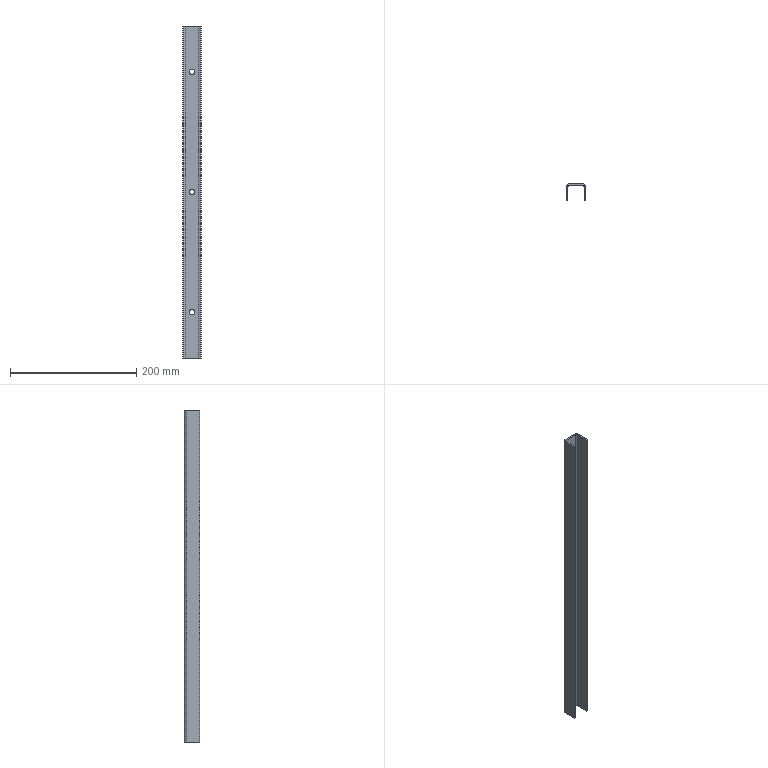Part | STEP file | SYL_0392D6J1SYL0380DJ10-1341050 | 1 solid | 28 faces | box 30 x 25 x 525 mm | volume 76794 mm3 | plane 18 | cylinder 10 | commonest cylinder face diameters 8 x8 4 x2
STEP:
#1=CARTESIAN_POINT('',(0.,23.,-194.));
#2=VERTEX_POINT('',#1);
#3=CARTESIAN_POINT('',(0.,25.,-194.));
#4=VERTEX_POINT('',#3);
#5=CARTESIAN_POINT('',(0.,25.,-194.));
#6=DIRECTION('',(0.,1.,0.));
#7=VECTOR('',#6,1000.);
#8=LINE('',#5,#7);
#9=EDGE_CURVE('',#2,#4,#8,.T.);
#10=ORIENTED_EDGE('',*,*,#9,.F.);
#11=CARTESIAN_POINT('',(0.,23.,-186.));
#12=VERTEX_POINT('',#11);
#13=CARTESIAN_POINT('',(0.,23.,-190.));
#14=DIRECTION('',(0.,-1.,0.));
#15=DIRECTION('',(0.,0.,-1.));
#16=AXIS2_PLACEMENT_3D('',#13,#14,#15);
#17=CIRCLE('',#16,4.);
#18=EDGE_CURVE('',#2,#12,#17,.T.);
#19=ORIENTED_EDGE('',*,*,#18,.T.);
#20=CARTESIAN_POINT('',(0.,25.,-186.));
#21=VERTEX_POINT('',#20);
#22=CARTESIAN_POINT('',(0.,25.,-186.));
#23=DIRECTION('',(0.,1.,0.));
#24=VECTOR('',#23,1000.);
#25=LINE('',#22,#24);
#26=EDGE_CURVE('',#12,#21,#25,.T.);
#27=ORIENTED_EDGE('',*,*,#26,.T.);
#28=CARTESIAN_POINT('',(0.,25.,-190.));
#29=DIRECTION('',(0.,-1.,0.));
#30=DIRECTION('',(0.,0.,-1.));
#31=AXIS2_PLACEMENT_3D('',#28,#29,#30);
#32=CIRCLE('',#31,4.);
#33=EDGE_CURVE('',#4,#21,#32,.T.);
#34=ORIENTED_EDGE('',*,*,#33,.F.);
#35=EDGE_LOOP('',(#10,#19,#27,#34));
#36=FACE_OUTER_BOUND('',#35,.T.);
#37=CARTESIAN_POINT('',(0.,25.,-190.));
#38=DIRECTION('',(0.,1.,0.));
#39=DIRECTION('',(0.,0.,1.));
#40=AXIS2_PLACEMENT_3D('',#37,#38,#39);
#41=CYLINDRICAL_SURFACE('',#40,4.);
#42=ADVANCED_FACE('',(#36),#41,.F.);
#43=CARTESIAN_POINT('',(0.,23.,-4.));
#44=VERTEX_POINT('',#43);
#45=CARTESIAN_POINT('',(0.,25.,-4.));
#46=VERTEX_POINT('',#45);
#47=CARTESIAN_POINT('',(0.,25.,-4.));
#48=DIRECTION('',(0.,1.,0.));
#49=VECTOR('',#48,1000.);
#50=LINE('',#47,#49);
#51=EDGE_CURVE('',#44,#46,#50,.T.);
#52=ORIENTED_EDGE('',*,*,#51,.F.);
#53=CARTESIAN_POINT('',(0.,23.,4.));
#54=VERTEX_POINT('',#53);
#55=CARTESIAN_POINT('',(0.,23.,0.));
#56=DIRECTION('',(0.,-1.,0.));
#57=DIRECTION('',(0.,0.,-1.));
#58=AXIS2_PLACEMENT_3D('',#55,#56,#57);
#59=CIRCLE('',#58,4.);
#60=EDGE_CURVE('',#44,#54,#59,.T.);
#61=ORIENTED_EDGE('',*,*,#60,.T.);
#62=CARTESIAN_POINT('',(0.,25.,4.));
#63=VERTEX_POINT('',#62);
#64=CARTESIAN_POINT('',(0.,25.,4.));
#65=DIRECTION('',(0.,1.,0.));
#66=VECTOR('',#65,1000.);
#67=LINE('',#64,#66);
#68=EDGE_CURVE('',#54,#63,#67,.T.);
#69=ORIENTED_EDGE('',*,*,#68,.T.);
#70=CARTESIAN_POINT('',(0.,25.,0.));
#71=DIRECTION('',(0.,-1.,0.));
#72=DIRECTION('',(0.,0.,-1.));
#73=AXIS2_PLACEMENT_3D('',#70,#71,#72);
#74=CIRCLE('',#73,4.);
#75=EDGE_CURVE('',#46,#63,#74,.T.);
#76=ORIENTED_EDGE('',*,*,#75,.F.);
#77=EDGE_LOOP('',(#52,#61,#69,#76));
#78=FACE_OUTER_BOUND('',#77,.T.);
#79=CARTESIAN_POINT('',(0.,25.,0.));
#80=DIRECTION('',(0.,1.,0.));
#81=DIRECTION('',(0.,0.,1.));
#82=AXIS2_PLACEMENT_3D('',#79,#80,#81);
#83=CYLINDRICAL_SURFACE('',#82,4.);
#84=ADVANCED_FACE('',(#78),#83,.F.);
#85=CARTESIAN_POINT('',(0.,23.,186.));
#86=VERTEX_POINT('',#85);
#87=CARTESIAN_POINT('',(0.,25.,186.));
#88=VERTEX_POINT('',#87);
#89=CARTESIAN_POINT('',(0.,25.,186.));
#90=DIRECTION('',(0.,1.,0.));
#91=VECTOR('',#90,1000.);
#92=LINE('',#89,#91);
#93=EDGE_CURVE('',#86,#88,#92,.T.);
#94=ORIENTED_EDGE('',*,*,#93,.F.);
#95=CARTESIAN_POINT('',(0.,23.,194.));
#96=VERTEX_POINT('',#95);
#97=CARTESIAN_POINT('',(0.,23.,190.));
#98=DIRECTION('',(0.,-1.,0.));
#99=DIRECTION('',(0.,0.,-1.));
#100=AXIS2_PLACEMENT_3D('',#97,#98,#99);
#101=CIRCLE('',#100,4.);
#102=EDGE_CURVE('',#86,#96,#101,.T.);
#103=ORIENTED_EDGE('',*,*,#102,.T.);
#104=CARTESIAN_POINT('',(0.,25.,194.));
#105=VERTEX_POINT('',#104);
#106=CARTESIAN_POINT('',(0.,25.,194.));
#107=DIRECTION('',(0.,1.,0.));
#108=VECTOR('',#107,1000.);
#109=LINE('',#106,#108);
#110=EDGE_CURVE('',#96,#105,#109,.T.);
#111=ORIENTED_EDGE('',*,*,#110,.T.);
#112=CARTESIAN_POINT('',(0.,25.,190.));
#113=DIRECTION('',(0.,-1.,0.));
#114=DIRECTION('',(0.,0.,-1.));
#115=AXIS2_PLACEMENT_3D('',#112,#113,#114);
#116=CIRCLE('',#115,4.);
#117=EDGE_CURVE('',#88,#105,#116,.T.);
#118=ORIENTED_EDGE('',*,*,#117,.F.);
#119=EDGE_LOOP('',(#94,#103,#111,#118));
#120=FACE_OUTER_BOUND('',#119,.T.);
#121=CARTESIAN_POINT('',(0.,25.,190.));
#122=DIRECTION('',(0.,1.,0.));
#123=DIRECTION('',(0.,0.,1.));
#124=AXIS2_PLACEMENT_3D('',#121,#122,#123);
#125=CYLINDRICAL_SURFACE('',#124,4.);
#126=ADVANCED_FACE('',(#120),#125,.F.);
#127=CARTESIAN_POINT('',(-11.,23.,-262.5));
#128=VERTEX_POINT('',#127);
#129=CARTESIAN_POINT('',(-11.,25.,-262.5));
#130=VERTEX_POINT('',#129);
#131=CARTESIAN_POINT('',(-11.,25.,-262.5));
#132=DIRECTION('',(0.,1.,0.));
#133=VECTOR('',#132,1000.);
#134=LINE('',#131,#133);
#135=EDGE_CURVE('',#128,#130,#134,.T.);
#136=ORIENTED_EDGE('',*,*,#135,.F.);
#137=CARTESIAN_POINT('',(-13.,21.,-262.5));
#138=VERTEX_POINT('',#137);
#139=CARTESIAN_POINT('',(-11.,21.,-262.5));
#140=DIRECTION('',(0.,0.,-1.));
#141=DIRECTION('',(1.,0.,0.));
#142=AXIS2_PLACEMENT_3D('',#139,#140,#141);
#143=CIRCLE('',#142,2.);
#144=EDGE_CURVE('',#138,#128,#143,.T.);
#145=ORIENTED_EDGE('',*,*,#144,.F.);
#146=CARTESIAN_POINT('',(-15.,21.,-262.5));
#147=VERTEX_POINT('',#146);
#148=CARTESIAN_POINT('',(-15.,21.,-262.5));
#149=DIRECTION('',(-1.,0.,0.));
#150=VECTOR('',#149,1000.);
#151=LINE('',#148,#150);
#152=EDGE_CURVE('',#138,#147,#151,.T.);
#153=ORIENTED_EDGE('',*,*,#152,.T.);
#154=CARTESIAN_POINT('',(-11.,21.,-262.5));
#155=DIRECTION('',(0.,0.,-1.));
#156=DIRECTION('',(-1.,0.,0.));
#157=AXIS2_PLACEMENT_3D('',#154,#155,#156);
#158=CIRCLE('',#157,4.);
#159=EDGE_CURVE('',#147,#130,#158,.T.);
#160=ORIENTED_EDGE('',*,*,#159,.T.);
#161=EDGE_LOOP('',(#136,#145,#153,#160));
#162=FACE_OUTER_BOUND('',#161,.T.);
#163=CARTESIAN_POINT('',(-11.,21.,-262.5));
#164=DIRECTION('',(0.,0.,1.));
#165=DIRECTION('',(1.,0.,0.));
#166=AXIS2_PLACEMENT_3D('',#163,#164,#165);
#167=PLANE('',#166);
#168=ADVANCED_FACE('',(#162),#167,.F.);
#169=ORIENTED_EDGE('',*,*,#152,.F.);
#170=CARTESIAN_POINT('',(-13.,0.,-262.5));
#171=VERTEX_POINT('',#170);
#172=CARTESIAN_POINT('',(-13.,21.,-262.5));
#173=DIRECTION('',(0.,-1.,0.));
#174=VECTOR('',#173,1000.);
#175=LINE('',#172,#174);
#176=EDGE_CURVE('',#138,#171,#175,.T.);
#177=ORIENTED_EDGE('',*,*,#176,.T.);
#178=CARTESIAN_POINT('',(-15.,0.,-262.5));
#179=VERTEX_POINT('',#178);
#180=CARTESIAN_POINT('',(-15.,0.,-262.5));
#181=DIRECTION('',(-1.,0.,0.));
#182=VECTOR('',#181,1000.);
#183=LINE('',#180,#182);
#184=EDGE_CURVE('',#171,#179,#183,.T.);
#185=ORIENTED_EDGE('',*,*,#184,.T.);
#186=CARTESIAN_POINT('',(-15.,21.,-262.5));
#187=DIRECTION('',(0.,-1.,0.));
#188=VECTOR('',#187,1000.);
#189=LINE('',#186,#188);
#190=EDGE_CURVE('',#147,#179,#189,.T.);
#191=ORIENTED_EDGE('',*,*,#190,.F.);
#192=EDGE_LOOP('',(#169,#177,#185,#191));
#193=FACE_OUTER_BOUND('',#192,.T.);
#194=CARTESIAN_POINT('',(-15.,21.,-262.5));
#195=DIRECTION('',(0.,0.,-1.));
#196=DIRECTION('',(0.,-1.,0.));
#197=AXIS2_PLACEMENT_3D('',#194,#195,#196);
#198=PLANE('',#197);
#199=ADVANCED_FACE('',(#193),#198,.T.);
#200=ORIENTED_EDGE('',*,*,#184,.F.);
#201=CARTESIAN_POINT('',(-13.,0.,262.5));
#202=VERTEX_POINT('',#201);
#203=CARTESIAN_POINT('',(-13.,0.,-262.5));
#204=DIRECTION('',(0.,0.,1.));
#205=VECTOR('',#204,1000.);
#206=LINE('',#203,#205);
#207=EDGE_CURVE('',#171,#202,#206,.T.);
#208=ORIENTED_EDGE('',*,*,#207,.T.);
#209=CARTESIAN_POINT('',(-15.,0.,262.5));
#210=VERTEX_POINT('',#209);
#211=CARTESIAN_POINT('',(-15.,0.,262.5));
#212=DIRECTION('',(-1.,0.,0.));
#213=VECTOR('',#212,1000.);
#214=LINE('',#211,#213);
#215=EDGE_CURVE('',#202,#210,#214,.T.);
#216=ORIENTED_EDGE('',*,*,#215,.T.);
#217=CARTESIAN_POINT('',(-15.,0.,-262.5));
#218=DIRECTION('',(0.,0.,1.));
#219=VECTOR('',#218,1000.);
#220=LINE('',#217,#219);
#221=EDGE_CURVE('',#179,#210,#220,.T.);
#222=ORIENTED_EDGE('',*,*,#221,.F.);
#223=EDGE_LOOP('',(#200,#208,#216,#222));
#224=FACE_OUTER_BOUND('',#223,.T.);
#225=CARTESIAN_POINT('',(-15.,0.,-262.5));
#226=DIRECTION('',(0.,-1.,0.));
#227=DIRECTION('',(0.,0.,1.));
#228=AXIS2_PLACEMENT_3D('',#225,#226,#227);
#229=PLANE('',#228);
#230=ADVANCED_FACE('',(#224),#229,.T.);
#231=ORIENTED_EDGE('',*,*,#215,.F.);
#232=CARTESIAN_POINT('',(-13.,21.,262.5));
#233=VERTEX_POINT('',#232);
#234=CARTESIAN_POINT('',(-13.,21.,262.5));
#235=DIRECTION('',(0.,-1.,0.));
#236=VECTOR('',#235,1000.);
#237=LINE('',#234,#236);
#238=EDGE_CURVE('',#233,#202,#237,.T.);
#239=ORIENTED_EDGE('',*,*,#238,.F.);
#240=CARTESIAN_POINT('',(-15.,21.,262.5));
#241=VERTEX_POINT('',#240);
#242=CARTESIAN_POINT('',(-15.,21.,262.5));
#243=DIRECTION('',(-1.,0.,0.));
#244=VECTOR('',#243,1000.);
#245=LINE('',#242,#244);
#246=EDGE_CURVE('',#233,#241,#245,.T.);
#247=ORIENTED_EDGE('',*,*,#246,.T.);
#248=CARTESIAN_POINT('',(-15.,21.,262.5));
#249=DIRECTION('',(0.,-1.,0.));
#250=VECTOR('',#249,1000.);
#251=LINE('',#248,#250);
#252=EDGE_CURVE('',#241,#210,#251,.T.);
#253=ORIENTED_EDGE('',*,*,#252,.T.);
#254=EDGE_LOOP('',(#231,#239,#247,#253));
#255=FACE_OUTER_BOUND('',#254,.T.);
#256=CARTESIAN_POINT('',(-15.,21.,262.5));
#257=DIRECTION('',(0.,0.,-1.));
#258=DIRECTION('',(0.,-1.,0.));
#259=AXIS2_PLACEMENT_3D('',#256,#257,#258);
#260=PLANE('',#259);
#261=ADVANCED_FACE('',(#255),#260,.F.);
#262=ORIENTED_EDGE('',*,*,#246,.F.);
#263=CARTESIAN_POINT('',(-11.,23.,262.5));
#264=VERTEX_POINT('',#263);
#265=CARTESIAN_POINT('',(-11.,21.,262.5));
#266=DIRECTION('',(0.,0.,1.));
#267=DIRECTION('',(1.,0.,0.));
#268=AXIS2_PLACEMENT_3D('',#265,#266,#267);
#269=CIRCLE('',#268,2.);
#270=EDGE_CURVE('',#264,#233,#269,.T.);
#271=ORIENTED_EDGE('',*,*,#270,.F.);
#272=CARTESIAN_POINT('',(-11.,25.,262.5));
#273=VERTEX_POINT('',#272);
#274=CARTESIAN_POINT('',(-11.,25.,262.5));
#275=DIRECTION('',(0.,1.,0.));
#276=VECTOR('',#275,1000.);
#277=LINE('',#274,#276);
#278=EDGE_CURVE('',#264,#273,#277,.T.);
#279=ORIENTED_EDGE('',*,*,#278,.T.);
#280=CARTESIAN_POINT('',(-11.,21.,262.5));
#281=DIRECTION('',(0.,0.,1.));
#282=DIRECTION('',(0.,1.,0.));
#283=AXIS2_PLACEMENT_3D('',#280,#281,#282);
#284=CIRCLE('',#283,4.);
#285=EDGE_CURVE('',#273,#241,#284,.T.);
#286=ORIENTED_EDGE('',*,*,#285,.T.);
#287=EDGE_LOOP('',(#262,#271,#279,#286));
#288=FACE_OUTER_BOUND('',#287,.T.);
#289=CARTESIAN_POINT('',(-11.,21.,262.5));
#290=DIRECTION('',(0.,0.,-1.));
#291=DIRECTION('',(-1.,0.,0.));
#292=AXIS2_PLACEMENT_3D('',#289,#290,#291);
#293=PLANE('',#292);
#294=ADVANCED_FACE('',(#288),#293,.F.);
#295=ORIENTED_EDGE('',*,*,#278,.F.);
#296=CARTESIAN_POINT('',(11.,23.,262.5));
#297=VERTEX_POINT('',#296);
#298=CARTESIAN_POINT('',(11.,23.,262.5));
#299=DIRECTION('',(-1.,0.,0.));
#300=VECTOR('',#299,1000.);
#301=LINE('',#298,#300);
#302=EDGE_CURVE('',#297,#264,#301,.T.);
#303=ORIENTED_EDGE('',*,*,#302,.F.);
#304=CARTESIAN_POINT('',(11.,25.,262.5));
#305=VERTEX_POINT('',#304);
#306=CARTESIAN_POINT('',(11.,25.,262.5));
#307=DIRECTION('',(0.,1.,0.));
#308=VECTOR('',#307,1000.);
#309=LINE('',#306,#308);
#310=EDGE_CURVE('',#297,#305,#309,.T.);
#311=ORIENTED_EDGE('',*,*,#310,.T.);
#312=CARTESIAN_POINT('',(11.,25.,262.5));
#313=DIRECTION('',(-1.,0.,0.));
#314=VECTOR('',#313,1000.);
#315=LINE('',#312,#314);
#316=EDGE_CURVE('',#305,#273,#315,.T.);
#317=ORIENTED_EDGE('',*,*,#316,.T.);
#318=EDGE_LOOP('',(#295,#303,#311,#317));
#319=FACE_OUTER_BOUND('',#318,.T.);
#320=CARTESIAN_POINT('',(11.,25.,262.5));
#321=DIRECTION('',(0.,0.,-1.));
#322=DIRECTION('',(-1.,0.,0.));
#323=AXIS2_PLACEMENT_3D('',#320,#321,#322);
#324=PLANE('',#323);
#325=ADVANCED_FACE('',(#319),#324,.F.);
#326=ORIENTED_EDGE('',*,*,#310,.F.);
#327=CARTESIAN_POINT('',(13.,21.,262.5));
#328=VERTEX_POINT('',#327);
#329=CARTESIAN_POINT('',(11.,21.,262.5));
#330=DIRECTION('',(0.,0.,1.));
#331=DIRECTION('',(1.,0.,0.));
#332=AXIS2_PLACEMENT_3D('',#329,#330,#331);
#333=CIRCLE('',#332,2.);
#334=EDGE_CURVE('',#328,#297,#333,.T.);
#335=ORIENTED_EDGE('',*,*,#334,.F.);
#336=CARTESIAN_POINT('',(15.,21.,262.5));
#337=VERTEX_POINT('',#336);
#338=CARTESIAN_POINT('',(15.,21.,262.5));
#339=DIRECTION('',(1.,0.,0.));
#340=VECTOR('',#339,1000.);
#341=LINE('',#338,#340);
#342=EDGE_CURVE('',#328,#337,#341,.T.);
#343=ORIENTED_EDGE('',*,*,#342,.T.);
#344=CARTESIAN_POINT('',(11.,21.,262.5));
#345=DIRECTION('',(0.,0.,1.));
#346=DIRECTION('',(1.,0.,0.));
#347=AXIS2_PLACEMENT_3D('',#344,#345,#346);
#348=CIRCLE('',#347,4.);
#349=EDGE_CURVE('',#337,#305,#348,.T.);
#350=ORIENTED_EDGE('',*,*,#349,.T.);
#351=EDGE_LOOP('',(#326,#335,#343,#350));
#352=FACE_OUTER_BOUND('',#351,.T.);
#353=CARTESIAN_POINT('',(11.,21.,262.5));
#354=DIRECTION('',(0.,0.,-1.));
#355=DIRECTION('',(-1.,0.,0.));
#356=AXIS2_PLACEMENT_3D('',#353,#354,#355);
#357=PLANE('',#356);
#358=ADVANCED_FACE('',(#352),#357,.F.);
#359=ORIENTED_EDGE('',*,*,#342,.F.);
#360=CARTESIAN_POINT('',(13.,0.,262.5));
#361=VERTEX_POINT('',#360);
#362=CARTESIAN_POINT('',(13.,0.,262.5));
#363=DIRECTION('',(0.,1.,0.));
#364=VECTOR('',#363,1000.);
#365=LINE('',#362,#364);
#366=EDGE_CURVE('',#361,#328,#365,.T.);
#367=ORIENTED_EDGE('',*,*,#366,.F.);
#368=CARTESIAN_POINT('',(15.,0.,262.5));
#369=VERTEX_POINT('',#368);
#370=CARTESIAN_POINT('',(15.,0.,262.5));
#371=DIRECTION('',(1.,0.,0.));
#372=VECTOR('',#371,1000.);
#373=LINE('',#370,#372);
#374=EDGE_CURVE('',#361,#369,#373,.T.);
#375=ORIENTED_EDGE('',*,*,#374,.T.);
#376=CARTESIAN_POINT('',(15.,0.,262.5));
#377=DIRECTION('',(0.,1.,0.));
#378=VECTOR('',#377,1000.);
#379=LINE('',#376,#378);
#380=EDGE_CURVE('',#369,#337,#379,.T.);
#381=ORIENTED_EDGE('',*,*,#380,.T.);
#382=EDGE_LOOP('',(#359,#367,#375,#381));
#383=FACE_OUTER_BOUND('',#382,.T.);
#384=CARTESIAN_POINT('',(15.,0.,262.5));
#385=DIRECTION('',(0.,0.,-1.));
#386=DIRECTION('',(0.,1.,0.));
#387=AXIS2_PLACEMENT_3D('',#384,#385,#386);
#388=PLANE('',#387);
#389=ADVANCED_FACE('',(#383),#388,.F.);
#390=ORIENTED_EDGE('',*,*,#374,.F.);
#391=CARTESIAN_POINT('',(13.,0.,-262.5));
#392=VERTEX_POINT('',#391);
#393=CARTESIAN_POINT('',(13.,0.,-262.5));
#394=DIRECTION('',(0.,0.,1.));
#395=VECTOR('',#394,1000.);
#396=LINE('',#393,#395);
#397=EDGE_CURVE('',#392,#361,#396,.T.);
#398=ORIENTED_EDGE('',*,*,#397,.F.);
#399=CARTESIAN_POINT('',(15.,0.,-262.5));
#400=VERTEX_POINT('',#399);
#401=CARTESIAN_POINT('',(15.,0.,-262.5));
#402=DIRECTION('',(1.,0.,0.));
#403=VECTOR('',#402,1000.);
#404=LINE('',#401,#403);
#405=EDGE_CURVE('',#392,#400,#404,.T.);
#406=ORIENTED_EDGE('',*,*,#405,.T.);
#407=CARTESIAN_POINT('',(15.,0.,-262.5));
#408=DIRECTION('',(0.,0.,1.));
#409=VECTOR('',#408,1000.);
#410=LINE('',#407,#409);
#411=EDGE_CURVE('',#400,#369,#410,.T.);
#412=ORIENTED_EDGE('',*,*,#411,.T.);
#413=EDGE_LOOP('',(#390,#398,#406,#412));
#414=FACE_OUTER_BOUND('',#413,.T.);
#415=CARTESIAN_POINT('',(15.,0.,-262.5));
#416=DIRECTION('',(0.,1.,0.));
#417=DIRECTION('',(0.,0.,1.));
#418=AXIS2_PLACEMENT_3D('',#415,#416,#417);
#419=PLANE('',#418);
#420=ADVANCED_FACE('',(#414),#419,.F.);
#421=ORIENTED_EDGE('',*,*,#405,.F.);
#422=CARTESIAN_POINT('',(13.,21.,-262.5));
#423=VERTEX_POINT('',#422);
#424=CARTESIAN_POINT('',(13.,0.,-262.5));
#425=DIRECTION('',(0.,1.,0.));
#426=VECTOR('',#425,1000.);
#427=LINE('',#424,#426);
#428=EDGE_CURVE('',#392,#423,#427,.T.);
#429=ORIENTED_EDGE('',*,*,#428,.T.);
#430=CARTESIAN_POINT('',(15.,21.,-262.5));
#431=VERTEX_POINT('',#430);
#432=CARTESIAN_POINT('',(15.,21.,-262.5));
#433=DIRECTION('',(1.,0.,0.));
#434=VECTOR('',#433,1000.);
#435=LINE('',#432,#434);
#436=EDGE_CURVE('',#423,#431,#435,.T.);
#437=ORIENTED_EDGE('',*,*,#436,.T.);
#438=CARTESIAN_POINT('',(15.,0.,-262.5));
#439=DIRECTION('',(0.,1.,0.));
#440=VECTOR('',#439,1000.);
#441=LINE('',#438,#440);
#442=EDGE_CURVE('',#400,#431,#441,.T.);
#443=ORIENTED_EDGE('',*,*,#442,.F.);
#444=EDGE_LOOP('',(#421,#429,#437,#443));
#445=FACE_OUTER_BOUND('',#444,.T.);
#446=CARTESIAN_POINT('',(15.,0.,-262.5));
#447=DIRECTION('',(0.,0.,-1.));
#448=DIRECTION('',(0.,1.,0.));
#449=AXIS2_PLACEMENT_3D('',#446,#447,#448);
#450=PLANE('',#449);
#451=ADVANCED_FACE('',(#445),#450,.T.);
#452=ORIENTED_EDGE('',*,*,#436,.F.);
#453=CARTESIAN_POINT('',(11.,23.,-262.5));
#454=VERTEX_POINT('',#453);
#455=CARTESIAN_POINT('',(11.,21.,-262.5));
#456=DIRECTION('',(0.,0.,-1.));
#457=DIRECTION('',(1.,0.,0.));
#458=AXIS2_PLACEMENT_3D('',#455,#456,#457);
#459=CIRCLE('',#458,2.);
#460=EDGE_CURVE('',#454,#423,#459,.T.);
#461=ORIENTED_EDGE('',*,*,#460,.F.);
#462=CARTESIAN_POINT('',(11.,25.,-262.5));
#463=VERTEX_POINT('',#462);
#464=CARTESIAN_POINT('',(11.,25.,-262.5));
#465=DIRECTION('',(0.,1.,0.));
#466=VECTOR('',#465,1000.);
#467=LINE('',#464,#466);
#468=EDGE_CURVE('',#454,#463,#467,.T.);
#469=ORIENTED_EDGE('',*,*,#468,.T.);
#470=CARTESIAN_POINT('',(11.,21.,-262.5));
#471=DIRECTION('',(0.,0.,-1.));
#472=DIRECTION('',(0.,1.,0.));
#473=AXIS2_PLACEMENT_3D('',#470,#471,#472);
#474=CIRCLE('',#473,4.);
#475=EDGE_CURVE('',#463,#431,#474,.T.);
#476=ORIENTED_EDGE('',*,*,#475,.T.);
#477=EDGE_LOOP('',(#452,#461,#469,#476));
#478=FACE_OUTER_BOUND('',#477,.T.);
#479=CARTESIAN_POINT('',(11.,21.,-262.5));
#480=DIRECTION('',(0.,0.,1.));
#481=DIRECTION('',(1.,0.,0.));
#482=AXIS2_PLACEMENT_3D('',#479,#480,#481);
#483=PLANE('',#482);
#484=ADVANCED_FACE('',(#478),#483,.F.);
#485=CARTESIAN_POINT('',(0.,23.,190.));
#486=DIRECTION('',(0.,-1.,0.));
#487=DIRECTION('',(0.,0.,-1.));
#488=AXIS2_PLACEMENT_3D('',#485,#486,#487);
#489=CIRCLE('',#488,4.);
#490=EDGE_CURVE('',#96,#86,#489,.T.);
#491=ORIENTED_EDGE('',*,*,#490,.T.);
#492=ORIENTED_EDGE('',*,*,#93,.T.);
#493=CARTESIAN_POINT('',(0.,25.,190.));
#494=DIRECTION('',(0.,-1.,0.));
#495=DIRECTION('',(0.,0.,1.));
#496=AXIS2_PLACEMENT_3D('',#493,#494,#495);
#497=CIRCLE('',#496,4.);
#498=EDGE_CURVE('',#105,#88,#497,.T.);
#499=ORIENTED_EDGE('',*,*,#498,.F.);
#500=ORIENTED_EDGE('',*,*,#110,.F.);
#501=EDGE_LOOP('',(#491,#492,#499,#500));
#502=FACE_OUTER_BOUND('',#501,.T.);
#503=CARTESIAN_POINT('',(0.,25.,190.));
#504=DIRECTION('',(0.,1.,0.));
#505=DIRECTION('',(0.,0.,1.));
#506=AXIS2_PLACEMENT_3D('',#503,#504,#505);
#507=CYLINDRICAL_SURFACE('',#506,4.);
#508=ADVANCED_FACE('',(#502),#507,.F.);
#509=CARTESIAN_POINT('',(0.,23.,0.));
#510=DIRECTION('',(0.,-1.,0.));
#511=DIRECTION('',(0.,0.,-1.));
#512=AXIS2_PLACEMENT_3D('',#509,#510,#511);
#513=CIRCLE('',#512,4.);
#514=EDGE_CURVE('',#54,#44,#513,.T.);
#515=ORIENTED_EDGE('',*,*,#514,.T.);
#516=ORIENTED_EDGE('',*,*,#51,.T.);
#517=CARTESIAN_POINT('',(0.,25.,0.));
#518=DIRECTION('',(0.,-1.,0.));
#519=DIRECTION('',(0.,0.,1.));
#520=AXIS2_PLACEMENT_3D('',#517,#518,#519);
#521=CIRCLE('',#520,4.);
#522=EDGE_CURVE('',#63,#46,#521,.T.);
#523=ORIENTED_EDGE('',*,*,#522,.F.);
#524=ORIENTED_EDGE('',*,*,#68,.F.);
#525=EDGE_LOOP('',(#515,#516,#523,#524));
#526=FACE_OUTER_BOUND('',#525,.T.);
#527=CARTESIAN_POINT('',(0.,25.,0.));
#528=DIRECTION('',(0.,1.,0.));
#529=DIRECTION('',(0.,0.,1.));
#530=AXIS2_PLACEMENT_3D('',#527,#528,#529);
#531=CYLINDRICAL_SURFACE('',#530,4.);
#532=ADVANCED_FACE('',(#526),#531,.F.);
#533=CARTESIAN_POINT('',(0.,23.,-190.));
#534=DIRECTION('',(0.,-1.,0.));
#535=DIRECTION('',(0.,0.,-1.));
#536=AXIS2_PLACEMENT_3D('',#533,#534,#535);
#537=CIRCLE('',#536,4.);
#538=EDGE_CURVE('',#12,#2,#537,.T.);
#539=ORIENTED_EDGE('',*,*,#538,.T.);
#540=ORIENTED_EDGE('',*,*,#9,.T.);
#541=CARTESIAN_POINT('',(0.,25.,-190.));
#542=DIRECTION('',(0.,-1.,0.));
#543=DIRECTION('',(0.,0.,1.));
#544=AXIS2_PLACEMENT_3D('',#541,#542,#543);
#545=CIRCLE('',#544,4.);
#546=EDGE_CURVE('',#21,#4,#545,.T.);
#547=ORIENTED_EDGE('',*,*,#546,.F.);
#548=ORIENTED_EDGE('',*,*,#26,.F.);
#549=EDGE_LOOP('',(#539,#540,#547,#548));
#550=FACE_OUTER_BOUND('',#549,.T.);
#551=CARTESIAN_POINT('',(0.,25.,-190.));
#552=DIRECTION('',(0.,1.,0.));
#553=DIRECTION('',(0.,0.,1.));
#554=AXIS2_PLACEMENT_3D('',#551,#552,#553);
#555=CYLINDRICAL_SURFACE('',#554,4.);
#556=ADVANCED_FACE('',(#550),#555,.F.);
#557=CARTESIAN_POINT('',(11.,23.,-262.5));
#558=DIRECTION('',(-1.,0.,0.));
#559=VECTOR('',#558,1000.);
#560=LINE('',#557,#559);
#561=EDGE_CURVE('',#454,#128,#560,.T.);
#562=ORIENTED_EDGE('',*,*,#561,.T.);
#563=ORIENTED_EDGE('',*,*,#135,.T.);
#564=CARTESIAN_POINT('',(11.,25.,-262.5));
#565=DIRECTION('',(-1.,0.,0.));
#566=VECTOR('',#565,1000.);
#567=LINE('',#564,#566);
#568=EDGE_CURVE('',#463,#130,#567,.T.);
#569=ORIENTED_EDGE('',*,*,#568,.F.);
#570=ORIENTED_EDGE('',*,*,#468,.F.);
#571=EDGE_LOOP('',(#562,#563,#569,#570));
#572=FACE_OUTER_BOUND('',#571,.T.);
#573=CARTESIAN_POINT('',(11.,25.,-262.5));
#574=DIRECTION('',(0.,0.,-1.));
#575=DIRECTION('',(-1.,0.,0.));
#576=AXIS2_PLACEMENT_3D('',#573,#574,#575);
#577=PLANE('',#576);
#578=ADVANCED_FACE('',(#572),#577,.T.);
#579=ORIENTED_EDGE('',*,*,#475,.F.);
#580=CARTESIAN_POINT('',(11.,25.,-262.5));
#581=DIRECTION('',(0.,0.,1.));
#582=VECTOR('',#581,1000.);
#583=LINE('',#580,#582);
#584=EDGE_CURVE('',#463,#305,#583,.T.);
#585=ORIENTED_EDGE('',*,*,#584,.T.);
#586=ORIENTED_EDGE('',*,*,#349,.F.);
#587=CARTESIAN_POINT('',(15.,21.,262.5));
#588=DIRECTION('',(0.,0.,-1.));
#589=VECTOR('',#588,1000.);
#590=LINE('',#587,#589);
#591=EDGE_CURVE('',#337,#431,#590,.T.);
#592=ORIENTED_EDGE('',*,*,#591,.T.);
#593=EDGE_LOOP('',(#579,#585,#586,#592));
#594=FACE_OUTER_BOUND('',#593,.T.);
#595=CARTESIAN_POINT('',(11.,21.,-262.5));
#596=DIRECTION('',(0.,0.,1.));
#597=DIRECTION('',(1.,0.,0.));
#598=AXIS2_PLACEMENT_3D('',#595,#596,#597);
#599=CYLINDRICAL_SURFACE('',#598,4.);
#600=ADVANCED_FACE('',(#594),#599,.T.);
#601=ORIENTED_EDGE('',*,*,#442,.T.);
#602=ORIENTED_EDGE('',*,*,#591,.F.);
#603=ORIENTED_EDGE('',*,*,#380,.F.);
#604=ORIENTED_EDGE('',*,*,#411,.F.);
#605=EDGE_LOOP('',(#601,#602,#603,#604));
#606=FACE_OUTER_BOUND('',#605,.T.);
#607=CARTESIAN_POINT('',(15.,0.,-262.5));
#608=DIRECTION('',(1.,0.,0.));
#609=DIRECTION('',(0.,1.,0.));
#610=AXIS2_PLACEMENT_3D('',#607,#608,#609);
#611=PLANE('',#610);
#612=ADVANCED_FACE('',(#606),#611,.T.);
#613=ORIENTED_EDGE('',*,*,#159,.F.);
#614=CARTESIAN_POINT('',(-15.,21.,-262.5));
#615=DIRECTION('',(0.,0.,1.));
#616=VECTOR('',#615,1000.);
#617=LINE('',#614,#616);
#618=EDGE_CURVE('',#147,#241,#617,.T.);
#619=ORIENTED_EDGE('',*,*,#618,.T.);
#620=ORIENTED_EDGE('',*,*,#285,.F.);
#621=CARTESIAN_POINT('',(-11.,25.,262.5));
#622=DIRECTION('',(0.,0.,-1.));
#623=VECTOR('',#622,1000.);
#624=LINE('',#621,#623);
#625=EDGE_CURVE('',#273,#130,#624,.T.);
#626=ORIENTED_EDGE('',*,*,#625,.T.);
#627=EDGE_LOOP('',(#613,#619,#620,#626));
#628=FACE_OUTER_BOUND('',#627,.T.);
#629=CARTESIAN_POINT('',(-11.,21.,-262.5));
#630=DIRECTION('',(0.,0.,1.));
#631=DIRECTION('',(1.,0.,0.));
#632=AXIS2_PLACEMENT_3D('',#629,#630,#631);
#633=CYLINDRICAL_SURFACE('',#632,4.);
#634=ADVANCED_FACE('',(#628),#633,.T.);
#635=ORIENTED_EDGE('',*,*,#117,.T.);
#636=ORIENTED_EDGE('',*,*,#498,.T.);
#637=EDGE_LOOP('',(#635,#636));
#638=FACE_BOUND('',#637,.T.);
#639=ORIENTED_EDGE('',*,*,#75,.T.);
#640=ORIENTED_EDGE('',*,*,#522,.T.);
#641=EDGE_LOOP('',(#639,#640));
#642=FACE_BOUND('',#641,.T.);
#643=ORIENTED_EDGE('',*,*,#33,.T.);
#644=ORIENTED_EDGE('',*,*,#546,.T.);
#645=EDGE_LOOP('',(#643,#644));
#646=FACE_BOUND('',#645,.T.);
#647=ORIENTED_EDGE('',*,*,#568,.T.);
#648=ORIENTED_EDGE('',*,*,#625,.F.);
#649=ORIENTED_EDGE('',*,*,#316,.F.);
#650=ORIENTED_EDGE('',*,*,#584,.F.);
#651=EDGE_LOOP('',(#647,#648,#649,#650));
#652=FACE_OUTER_BOUND('',#651,.T.);
#653=CARTESIAN_POINT('',(11.,25.,-262.5));
#654=DIRECTION('',(0.,1.,0.));
#655=DIRECTION('',(1.,0.,0.));
#656=AXIS2_PLACEMENT_3D('',#653,#654,#655);
#657=PLANE('',#656);
#658=ADVANCED_FACE('',(#638,#642,#646,#652),#657,.T.);
#659=ORIENTED_EDGE('',*,*,#190,.T.);
#660=ORIENTED_EDGE('',*,*,#221,.T.);
#661=ORIENTED_EDGE('',*,*,#252,.F.);
#662=ORIENTED_EDGE('',*,*,#618,.F.);
#663=EDGE_LOOP('',(#659,#660,#661,#662));
#664=FACE_OUTER_BOUND('',#663,.T.);
#665=CARTESIAN_POINT('',(-15.,21.,-262.5));
#666=DIRECTION('',(-1.,0.,0.));
#667=DIRECTION('',(0.,0.,1.));
#668=AXIS2_PLACEMENT_3D('',#665,#666,#667);
#669=PLANE('',#668);
#670=ADVANCED_FACE('',(#664),#669,.T.);
#671=ORIENTED_EDGE('',*,*,#460,.T.);
#672=CARTESIAN_POINT('',(13.,21.,-262.5));
#673=DIRECTION('',(0.,0.,-1.));
#674=VECTOR('',#673,1000.);
#675=LINE('',#672,#674);
#676=EDGE_CURVE('',#328,#423,#675,.T.);
#677=ORIENTED_EDGE('',*,*,#676,.F.);
#678=ORIENTED_EDGE('',*,*,#334,.T.);
#679=CARTESIAN_POINT('',(11.,23.,-262.5));
#680=DIRECTION('',(0.,0.,1.));
#681=VECTOR('',#680,1000.);
#682=LINE('',#679,#681);
#683=EDGE_CURVE('',#454,#297,#682,.T.);
#684=ORIENTED_EDGE('',*,*,#683,.F.);
#685=EDGE_LOOP('',(#671,#677,#678,#684));
#686=FACE_OUTER_BOUND('',#685,.T.);
#687=CARTESIAN_POINT('',(11.,21.,-262.5));
#688=DIRECTION('',(0.,0.,1.));
#689=DIRECTION('',(1.,0.,0.));
#690=AXIS2_PLACEMENT_3D('',#687,#688,#689);
#691=CYLINDRICAL_SURFACE('',#690,2.);
#692=ADVANCED_FACE('',(#686),#691,.F.);
#693=ORIENTED_EDGE('',*,*,#428,.F.);
#694=ORIENTED_EDGE('',*,*,#397,.T.);
#695=ORIENTED_EDGE('',*,*,#366,.T.);
#696=ORIENTED_EDGE('',*,*,#676,.T.);
#697=EDGE_LOOP('',(#693,#694,#695,#696));
#698=FACE_OUTER_BOUND('',#697,.T.);
#699=CARTESIAN_POINT('',(13.,0.,-262.5));
#700=DIRECTION('',(1.,0.,0.));
#701=DIRECTION('',(0.,1.,0.));
#702=AXIS2_PLACEMENT_3D('',#699,#700,#701);
#703=PLANE('',#702);
#704=ADVANCED_FACE('',(#698),#703,.F.);
#705=ORIENTED_EDGE('',*,*,#144,.T.);
#706=CARTESIAN_POINT('',(-11.,23.,-262.5));
#707=DIRECTION('',(0.,0.,-1.));
#708=VECTOR('',#707,1000.);
#709=LINE('',#706,#708);
#710=EDGE_CURVE('',#264,#128,#709,.T.);
#711=ORIENTED_EDGE('',*,*,#710,.F.);
#712=ORIENTED_EDGE('',*,*,#270,.T.);
#713=CARTESIAN_POINT('',(-13.,21.,-262.5));
#714=DIRECTION('',(0.,0.,1.));
#715=VECTOR('',#714,1000.);
#716=LINE('',#713,#715);
#717=EDGE_CURVE('',#138,#233,#716,.T.);
#718=ORIENTED_EDGE('',*,*,#717,.F.);
#719=EDGE_LOOP('',(#705,#711,#712,#718));
#720=FACE_OUTER_BOUND('',#719,.T.);
#721=CARTESIAN_POINT('',(-11.,21.,-262.5));
#722=DIRECTION('',(0.,0.,1.));
#723=DIRECTION('',(1.,0.,0.));
#724=AXIS2_PLACEMENT_3D('',#721,#722,#723);
#725=CYLINDRICAL_SURFACE('',#724,2.);
#726=ADVANCED_FACE('',(#720),#725,.F.);
#727=ORIENTED_EDGE('',*,*,#102,.F.);
#728=ORIENTED_EDGE('',*,*,#490,.F.);
#729=EDGE_LOOP('',(#727,#728));
#730=FACE_BOUND('',#729,.T.);
#731=ORIENTED_EDGE('',*,*,#60,.F.);
#732=ORIENTED_EDGE('',*,*,#514,.F.);
#733=EDGE_LOOP('',(#731,#732));
#734=FACE_BOUND('',#733,.T.);
#735=ORIENTED_EDGE('',*,*,#18,.F.);
#736=ORIENTED_EDGE('',*,*,#538,.F.);
#737=EDGE_LOOP('',(#735,#736));
#738=FACE_BOUND('',#737,.T.);
#739=ORIENTED_EDGE('',*,*,#561,.F.);
#740=ORIENTED_EDGE('',*,*,#683,.T.);
#741=ORIENTED_EDGE('',*,*,#302,.T.);
#742=ORIENTED_EDGE('',*,*,#710,.T.);
#743=EDGE_LOOP('',(#739,#740,#741,#742));
#744=FACE_OUTER_BOUND('',#743,.T.);
#745=CARTESIAN_POINT('',(11.,23.,-262.5));
#746=DIRECTION('',(0.,1.,0.));
#747=DIRECTION('',(1.,0.,0.));
#748=AXIS2_PLACEMENT_3D('',#745,#746,#747);
#749=PLANE('',#748);
#750=ADVANCED_FACE('',(#730,#734,#738,#744),#749,.F.);
#751=ORIENTED_EDGE('',*,*,#176,.F.);
#752=ORIENTED_EDGE('',*,*,#717,.T.);
#753=ORIENTED_EDGE('',*,*,#238,.T.);
#754=ORIENTED_EDGE('',*,*,#207,.F.);
#755=EDGE_LOOP('',(#751,#752,#753,#754));
#756=FACE_OUTER_BOUND('',#755,.T.);
#757=CARTESIAN_POINT('',(-13.,21.,-262.5));
#758=DIRECTION('',(-1.,0.,0.));
#759=DIRECTION('',(0.,0.,1.));
#760=AXIS2_PLACEMENT_3D('',#757,#758,#759);
#761=PLANE('',#760);
#762=ADVANCED_FACE('',(#756),#761,.F.);
#763=CLOSED_SHELL('',(#42,#84,#126,#168,#199,#230,#261,#294,#325,#358,#389,#420,#451,#484,#508,#532,#556,#578,#600,#612,#634,#658,#670,#692,#704,#726,#750,#762));
#764=MANIFOLD_SOLID_BREP('',#763);
#765=CARTESIAN_POINT('',(0.,0.,0.));
#766=DIRECTION('',(0.,0.,1.));
#767=DIRECTION('',(1.,0.,0.));
#768=AXIS2_PLACEMENT_3D('',#765,#766,#767);
#769=(LENGTH_UNIT()NAMED_UNIT(*)SI_UNIT(.MILLI.,.METRE.));
#770=UNCERTAINTY_MEASURE_WITH_UNIT(LENGTH_MEASURE(0.00001),#769,'','');
#771=(NAMED_UNIT(*)PLANE_ANGLE_UNIT()SI_UNIT($,.RADIAN.));
#772=(NAMED_UNIT(*)SI_UNIT($,.STERADIAN.)SOLID_ANGLE_UNIT());
#773=(GEOMETRIC_REPRESENTATION_CONTEXT(3)GLOBAL_UNCERTAINTY_ASSIGNED_CONTEXT((#770))GLOBAL_UNIT_ASSIGNED_CONTEXT((#769,#771,#772))REPRESENTATION_CONTEXT('',''));
#774=ADVANCED_BREP_SHAPE_REPRESENTATION('',(#764,#768),#773);